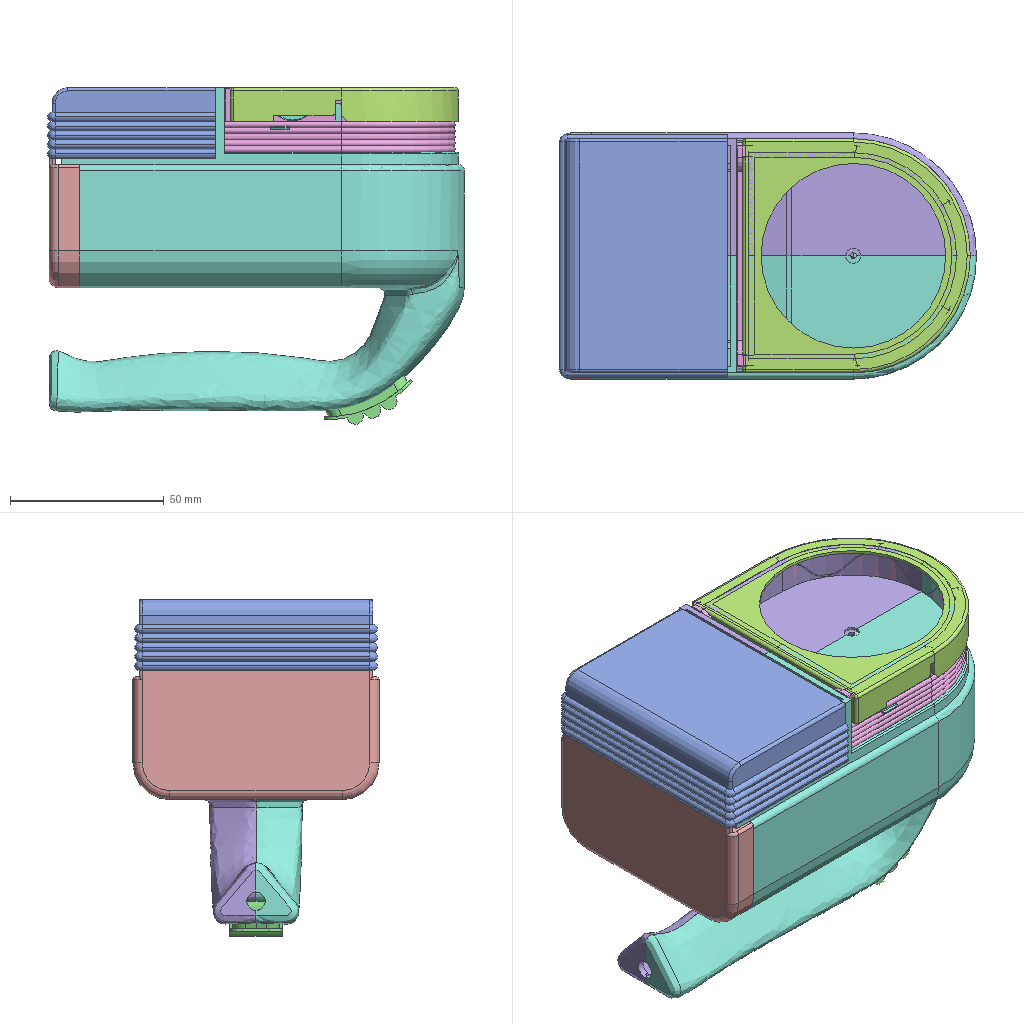Assembly | SolidWorks | 14 different items | 14 placed | box 135 x 80 x 109 mm
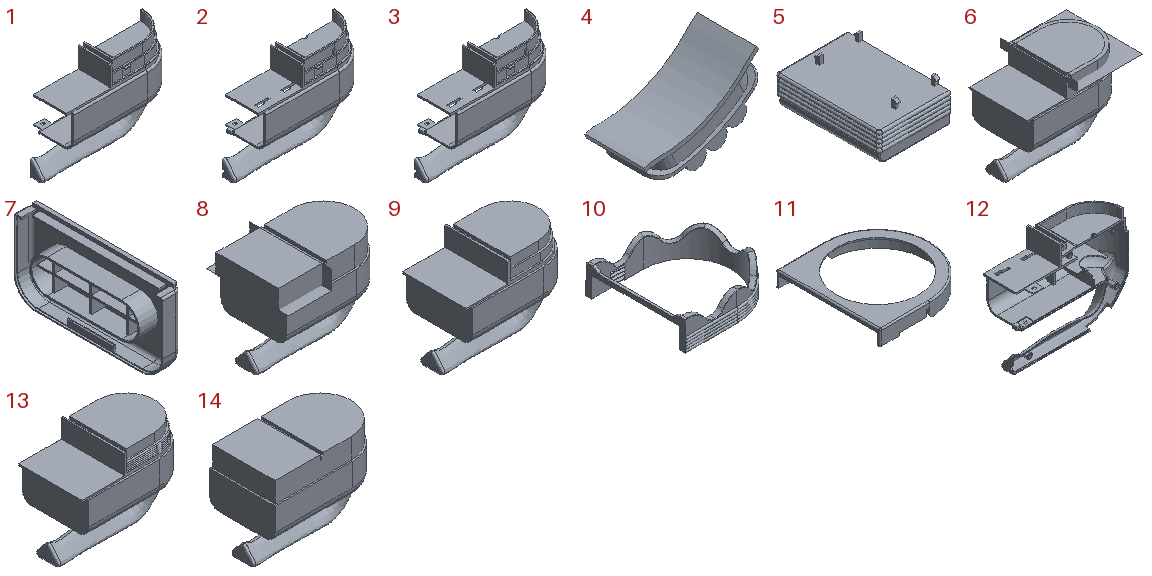Parts list (item | quantity | size | volume | features):
1 | x1 | 135 x 50.019 x 105.415 mm | 48449 mm3 | features ICE 9, Fillet 6, BossThin 3, CombineBodies 1, CompositeCurve 1, SewRefSurface 1, Shell 1, Stock 1, SurfCut 1, Sweep 1
2 | x1 | 135 x 50.019 x 105.415 mm | 49896 mm3 | features ICE 11, Fillet 1, LPattern 1, Rib 1, Stock 1
3 | x1 | 135 x 50.019 x 105.415 mm | 49896 mm3 | features Stock 1
4 | x1 | 32.392 x 17 x 20.411 mm | 3378 mm3 | features ICE 5, ExtruRefSurface 4, ExtendRefSurface 2, Fillet 2, Thicken 2, BossThin 1, CombineBodies 1, SewRefSurface 1, Shell 1, Stock 1, SurfCut 1, TrimRefSurface 1
5 | x1 | 54.5 x 79 x 28.958 mm | 25997 mm3 | features Chamfer 2, Fillet 2, ICE 2, LPattern 1, MirrorPattern 1, Shell 1, Stock 1, SurfCut 1, Sweep 1
6 | x1 | - | - | features ExtruRefSurface 2, SewRefSurface 1, Stock 1, SurfCut 1, TrimRefSurface 1
7 | x1 | 12 x 80 x 42 mm | 7212 mm3 | features BossThin 5, Fillet 4, ICE 3, FillRefSurface 1, SewRefSurface 1, Shell 1, Stock 1, SurfCut 1, SweepCut 1, TrimRefSurface 1
8 | x1 | - | - | features TrimRefSurface 3, ExtruRefSurface 1, Stock 1, SurfCut 1
9 | x1 | - | - | features ICE 1, SewRefSurface 1, Stock 1, SurfCut 1, TrimRefSurface 1
10 | x1 | 75 x 74 x 21 mm | 13589 mm3 | features ICE 8, Chamfer 3, ExtruRefSurface 2, Fillet 2, MirrorPattern 2, SurfCut 2, CurvePattern 1, LPattern 1, Stock 1
11 | x1 | 74 x 76 x 11 mm | 5943 mm3 | features ICE 8, Fillet 2, Chamfer 1, Stock 1, SurfCut 1
12 | x1 | 135 x 49.981 x 105.415 mm | 48344 mm3 | features ICE 24, Fillet 8, BossThin 4, CombineBodies 2, Rib 2, CompositeCurve 1, SewRefSurface 1, Shell 1, Stock 1, SurfCut 1, SweepCut 1
13 | x1 | - | - | features ExtruRefSurface 2, SurfCut 2, LPattern 1, SewRefSurface 1, Stock 1, Sweep 1, TrimRefSurface 1
14 | x1 | - | - | features ExtruRefSurface 3, FillRefSurface 3, Fillet 2, BlendRefSurface 1, DelFace 1, Extrusion 1, ICE 1, MirrorSolid 1, SewRefSurface 1, TrimRefSurface 1
Mates (type | each side: item.copy, entity, surface, feature):
Coincident | 9.1 face plane Level-4 Control | 7.1 face plane Level-1 Control | 2 times
Coincident | 9.1 face plane Level-4 Control | 7.1 face plane Boss-Extrude1
Coincident | 9.1 face plane Level-4 Control | 5.1 face plane Level-2 Control
Coincident | 9.1 face plane Boss-Extrude1 | 5.1 face plane Cut-with-Surface1
Width | 5.1 face plane Level-2 Control | 5.1 face plane Level-2 Control | 9.1 face plane Level-4 Control | 9.1 face plane Level-4 Control